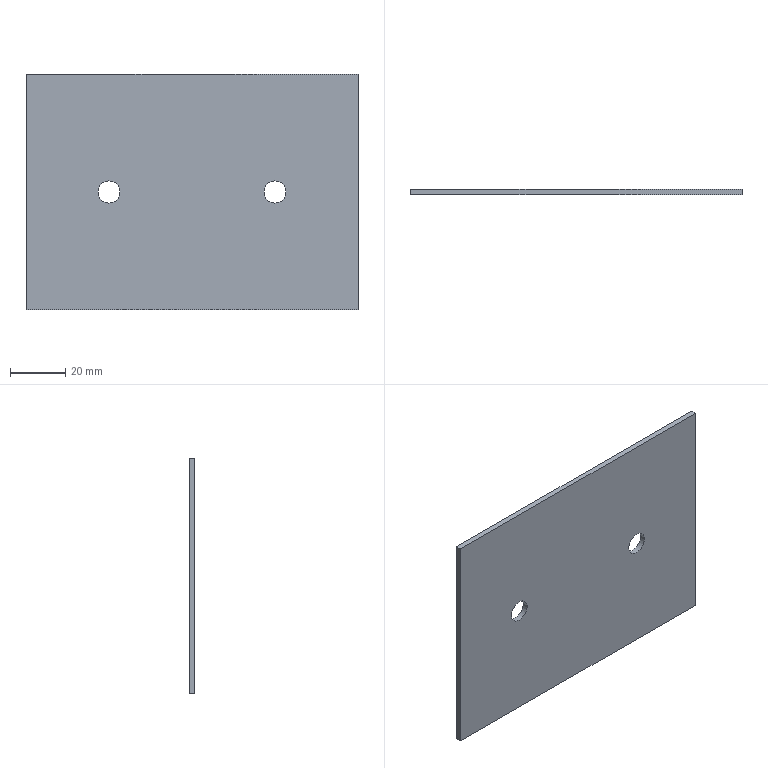Part | STEP file | JBJ-P-1003-05 | 1 solid | 8 faces | box 120 x 2 x 85 mm | volume 20199 mm3 | plane 6 | cylinder 2 | commonest cylinder face diameters 8 x2
STEP:
#1=CARTESIAN_POINT('',(0.,0.,0.));
#2=VERTEX_POINT('',#1);
#3=CARTESIAN_POINT('',(0.,0.,85.));
#4=VERTEX_POINT('',#3);
#5=CARTESIAN_POINT('',(0.,0.,0.));
#6=DIRECTION('',(0.,0.,1.));
#7=VECTOR('',#6,1000.);
#8=LINE('',#5,#7);
#9=EDGE_CURVE('',#2,#4,#8,.T.);
#10=ORIENTED_EDGE('',*,*,#9,.T.);
#11=CARTESIAN_POINT('',(0.,2.,85.));
#12=VERTEX_POINT('',#11);
#13=CARTESIAN_POINT('',(0.,2.,85.));
#14=DIRECTION('',(0.,-1.,0.));
#15=VECTOR('',#14,1000.);
#16=LINE('',#13,#15);
#17=EDGE_CURVE('',#12,#4,#16,.T.);
#18=ORIENTED_EDGE('',*,*,#17,.F.);
#19=CARTESIAN_POINT('',(0.,2.,0.));
#20=VERTEX_POINT('',#19);
#21=CARTESIAN_POINT('',(0.,2.,0.));
#22=DIRECTION('',(0.,0.,1.));
#23=VECTOR('',#22,1000.);
#24=LINE('',#21,#23);
#25=EDGE_CURVE('',#20,#12,#24,.T.);
#26=ORIENTED_EDGE('',*,*,#25,.F.);
#27=CARTESIAN_POINT('',(0.,2.,0.));
#28=DIRECTION('',(0.,-1.,0.));
#29=VECTOR('',#28,1000.);
#30=LINE('',#27,#29);
#31=EDGE_CURVE('',#20,#2,#30,.T.);
#32=ORIENTED_EDGE('',*,*,#31,.T.);
#33=EDGE_LOOP('',(#10,#18,#26,#32));
#34=FACE_OUTER_BOUND('',#33,.T.);
#35=CARTESIAN_POINT('',(0.,2.,0.));
#36=DIRECTION('',(1.,0.,0.));
#37=DIRECTION('',(0.,0.,-1.));
#38=AXIS2_PLACEMENT_3D('',#35,#36,#37);
#39=PLANE('',#38);
#40=ADVANCED_FACE('',(#34),#39,.F.);
#41=CARTESIAN_POINT('',(120.,0.,85.));
#42=VERTEX_POINT('',#41);
#43=CARTESIAN_POINT('',(0.,0.,85.));
#44=DIRECTION('',(1.,0.,0.));
#45=VECTOR('',#44,1000.);
#46=LINE('',#43,#45);
#47=EDGE_CURVE('',#4,#42,#46,.T.);
#48=ORIENTED_EDGE('',*,*,#47,.T.);
#49=CARTESIAN_POINT('',(120.,2.,85.));
#50=VERTEX_POINT('',#49);
#51=CARTESIAN_POINT('',(120.,2.,85.));
#52=DIRECTION('',(0.,-1.,0.));
#53=VECTOR('',#52,1000.);
#54=LINE('',#51,#53);
#55=EDGE_CURVE('',#50,#42,#54,.T.);
#56=ORIENTED_EDGE('',*,*,#55,.F.);
#57=CARTESIAN_POINT('',(0.,2.,85.));
#58=DIRECTION('',(1.,0.,0.));
#59=VECTOR('',#58,1000.);
#60=LINE('',#57,#59);
#61=EDGE_CURVE('',#12,#50,#60,.T.);
#62=ORIENTED_EDGE('',*,*,#61,.F.);
#63=ORIENTED_EDGE('',*,*,#17,.T.);
#64=EDGE_LOOP('',(#48,#56,#62,#63));
#65=FACE_OUTER_BOUND('',#64,.T.);
#66=CARTESIAN_POINT('',(0.,2.,85.));
#67=DIRECTION('',(0.,0.,-1.));
#68=DIRECTION('',(-1.,0.,0.));
#69=AXIS2_PLACEMENT_3D('',#66,#67,#68);
#70=PLANE('',#69);
#71=ADVANCED_FACE('',(#65),#70,.F.);
#72=CARTESIAN_POINT('',(120.,0.,0.));
#73=VERTEX_POINT('',#72);
#74=CARTESIAN_POINT('',(120.,0.,0.));
#75=DIRECTION('',(0.,0.,-1.));
#76=VECTOR('',#75,1000.);
#77=LINE('',#74,#76);
#78=EDGE_CURVE('',#42,#73,#77,.T.);
#79=ORIENTED_EDGE('',*,*,#78,.T.);
#80=CARTESIAN_POINT('',(120.,2.,0.));
#81=VERTEX_POINT('',#80);
#82=CARTESIAN_POINT('',(120.,2.,0.));
#83=DIRECTION('',(0.,-1.,0.));
#84=VECTOR('',#83,1000.);
#85=LINE('',#82,#84);
#86=EDGE_CURVE('',#81,#73,#85,.T.);
#87=ORIENTED_EDGE('',*,*,#86,.F.);
#88=CARTESIAN_POINT('',(120.,2.,0.));
#89=DIRECTION('',(0.,0.,-1.));
#90=VECTOR('',#89,1000.);
#91=LINE('',#88,#90);
#92=EDGE_CURVE('',#50,#81,#91,.T.);
#93=ORIENTED_EDGE('',*,*,#92,.F.);
#94=ORIENTED_EDGE('',*,*,#55,.T.);
#95=EDGE_LOOP('',(#79,#87,#93,#94));
#96=FACE_OUTER_BOUND('',#95,.T.);
#97=CARTESIAN_POINT('',(120.,2.,0.));
#98=DIRECTION('',(-1.,0.,0.));
#99=DIRECTION('',(0.,0.,1.));
#100=AXIS2_PLACEMENT_3D('',#97,#98,#99);
#101=PLANE('',#100);
#102=ADVANCED_FACE('',(#96),#101,.F.);
#103=CARTESIAN_POINT('',(0.,0.,0.));
#104=DIRECTION('',(-1.,0.,0.));
#105=VECTOR('',#104,1000.);
#106=LINE('',#103,#105);
#107=EDGE_CURVE('',#73,#2,#106,.T.);
#108=ORIENTED_EDGE('',*,*,#107,.T.);
#109=ORIENTED_EDGE('',*,*,#31,.F.);
#110=CARTESIAN_POINT('',(0.,2.,0.));
#111=DIRECTION('',(-1.,0.,0.));
#112=VECTOR('',#111,1000.);
#113=LINE('',#110,#112);
#114=EDGE_CURVE('',#81,#20,#113,.T.);
#115=ORIENTED_EDGE('',*,*,#114,.F.);
#116=ORIENTED_EDGE('',*,*,#86,.T.);
#117=EDGE_LOOP('',(#108,#109,#115,#116));
#118=FACE_OUTER_BOUND('',#117,.T.);
#119=CARTESIAN_POINT('',(0.,2.,0.));
#120=DIRECTION('',(0.,0.,1.));
#121=DIRECTION('',(1.,0.,0.));
#122=AXIS2_PLACEMENT_3D('',#119,#120,#121);
#123=PLANE('',#122);
#124=ADVANCED_FACE('',(#118),#123,.F.);
#125=CARTESIAN_POINT('',(90.,2.,46.5));
#126=VERTEX_POINT('',#125);
#127=CARTESIAN_POINT('',(90.,2.,42.5));
#128=DIRECTION('',(0.,1.,0.));
#129=DIRECTION('',(0.,0.,1.));
#130=AXIS2_PLACEMENT_3D('',#127,#128,#129);
#131=CIRCLE('',#130,4.);
#132=EDGE_CURVE('',#126,#126,#131,.T.);
#133=ORIENTED_EDGE('',*,*,#132,.F.);
#134=EDGE_LOOP('',(#133));
#135=FACE_BOUND('',#134,.T.);
#136=CARTESIAN_POINT('',(30.,2.,46.5));
#137=VERTEX_POINT('',#136);
#138=CARTESIAN_POINT('',(30.,2.,42.5));
#139=DIRECTION('',(0.,1.,0.));
#140=DIRECTION('',(0.,0.,1.));
#141=AXIS2_PLACEMENT_3D('',#138,#139,#140);
#142=CIRCLE('',#141,4.);
#143=EDGE_CURVE('',#137,#137,#142,.T.);
#144=ORIENTED_EDGE('',*,*,#143,.F.);
#145=EDGE_LOOP('',(#144));
#146=FACE_BOUND('',#145,.T.);
#147=ORIENTED_EDGE('',*,*,#25,.T.);
#148=ORIENTED_EDGE('',*,*,#61,.T.);
#149=ORIENTED_EDGE('',*,*,#92,.T.);
#150=ORIENTED_EDGE('',*,*,#114,.T.);
#151=EDGE_LOOP('',(#147,#148,#149,#150));
#152=FACE_OUTER_BOUND('',#151,.T.);
#153=CARTESIAN_POINT('',(0.,2.,0.));
#154=DIRECTION('',(0.,1.,0.));
#155=DIRECTION('',(0.,0.,1.));
#156=AXIS2_PLACEMENT_3D('',#153,#154,#155);
#157=PLANE('',#156);
#158=ADVANCED_FACE('',(#135,#146,#152),#157,.T.);
#159=CARTESIAN_POINT('',(90.,0.,46.5));
#160=VERTEX_POINT('',#159);
#161=CARTESIAN_POINT('',(90.,0.,42.5));
#162=DIRECTION('',(0.,1.,0.));
#163=DIRECTION('',(0.,0.,1.));
#164=AXIS2_PLACEMENT_3D('',#161,#162,#163);
#165=CIRCLE('',#164,4.);
#166=EDGE_CURVE('',#160,#160,#165,.T.);
#167=ORIENTED_EDGE('',*,*,#166,.T.);
#168=EDGE_LOOP('',(#167));
#169=FACE_BOUND('',#168,.T.);
#170=CARTESIAN_POINT('',(30.,0.,46.5));
#171=VERTEX_POINT('',#170);
#172=CARTESIAN_POINT('',(30.,0.,42.5));
#173=DIRECTION('',(0.,1.,0.));
#174=DIRECTION('',(0.,0.,1.));
#175=AXIS2_PLACEMENT_3D('',#172,#173,#174);
#176=CIRCLE('',#175,4.);
#177=EDGE_CURVE('',#171,#171,#176,.T.);
#178=ORIENTED_EDGE('',*,*,#177,.T.);
#179=EDGE_LOOP('',(#178));
#180=FACE_BOUND('',#179,.T.);
#181=ORIENTED_EDGE('',*,*,#9,.F.);
#182=ORIENTED_EDGE('',*,*,#107,.F.);
#183=ORIENTED_EDGE('',*,*,#78,.F.);
#184=ORIENTED_EDGE('',*,*,#47,.F.);
#185=EDGE_LOOP('',(#181,#182,#183,#184));
#186=FACE_OUTER_BOUND('',#185,.T.);
#187=CARTESIAN_POINT('',(0.,0.,0.));
#188=DIRECTION('',(0.,1.,0.));
#189=DIRECTION('',(0.,0.,1.));
#190=AXIS2_PLACEMENT_3D('',#187,#188,#189);
#191=PLANE('',#190);
#192=ADVANCED_FACE('',(#169,#180,#186),#191,.F.);
#193=ORIENTED_EDGE('',*,*,#177,.F.);
#194=EDGE_LOOP('',(#193));
#195=FACE_OUTER_BOUND('',#194,.T.);
#196=ORIENTED_EDGE('',*,*,#143,.T.);
#197=EDGE_LOOP('',(#196));
#198=FACE_OUTER_BOUND('',#197,.T.);
#199=CARTESIAN_POINT('',(30.,0.,42.5));
#200=DIRECTION('',(0.,1.,0.));
#201=DIRECTION('',(0.,0.,1.));
#202=AXIS2_PLACEMENT_3D('',#199,#200,#201);
#203=CYLINDRICAL_SURFACE('',#202,4.);
#204=ADVANCED_FACE('',(#195,#198),#203,.F.);
#205=ORIENTED_EDGE('',*,*,#166,.F.);
#206=EDGE_LOOP('',(#205));
#207=FACE_OUTER_BOUND('',#206,.T.);
#208=ORIENTED_EDGE('',*,*,#132,.T.);
#209=EDGE_LOOP('',(#208));
#210=FACE_OUTER_BOUND('',#209,.T.);
#211=CARTESIAN_POINT('',(90.,0.,42.5));
#212=DIRECTION('',(0.,1.,0.));
#213=DIRECTION('',(0.,0.,1.));
#214=AXIS2_PLACEMENT_3D('',#211,#212,#213);
#215=CYLINDRICAL_SURFACE('',#214,4.);
#216=ADVANCED_FACE('',(#207,#210),#215,.F.);
#217=CLOSED_SHELL('',(#40,#71,#102,#124,#158,#192,#204,#216));
#218=MANIFOLD_SOLID_BREP('',#217);
#219=CARTESIAN_POINT('',(0.,0.,0.));
#220=DIRECTION('',(0.,0.,1.));
#221=DIRECTION('',(1.,0.,0.));
#222=AXIS2_PLACEMENT_3D('',#219,#220,#221);
#223=(LENGTH_UNIT()NAMED_UNIT(*)SI_UNIT(.MILLI.,.METRE.));
#224=UNCERTAINTY_MEASURE_WITH_UNIT(LENGTH_MEASURE(0.00001),#223,'','');
#225=(NAMED_UNIT(*)PLANE_ANGLE_UNIT()SI_UNIT($,.RADIAN.));
#226=(NAMED_UNIT(*)SI_UNIT($,.STERADIAN.)SOLID_ANGLE_UNIT());
#227=(GEOMETRIC_REPRESENTATION_CONTEXT(3)GLOBAL_UNCERTAINTY_ASSIGNED_CONTEXT((#224))GLOBAL_UNIT_ASSIGNED_CONTEXT((#223,#225,#226))REPRESENTATION_CONTEXT('',''));
#228=ADVANCED_BREP_SHAPE_REPRESENTATION('',(#218,#222),#227);